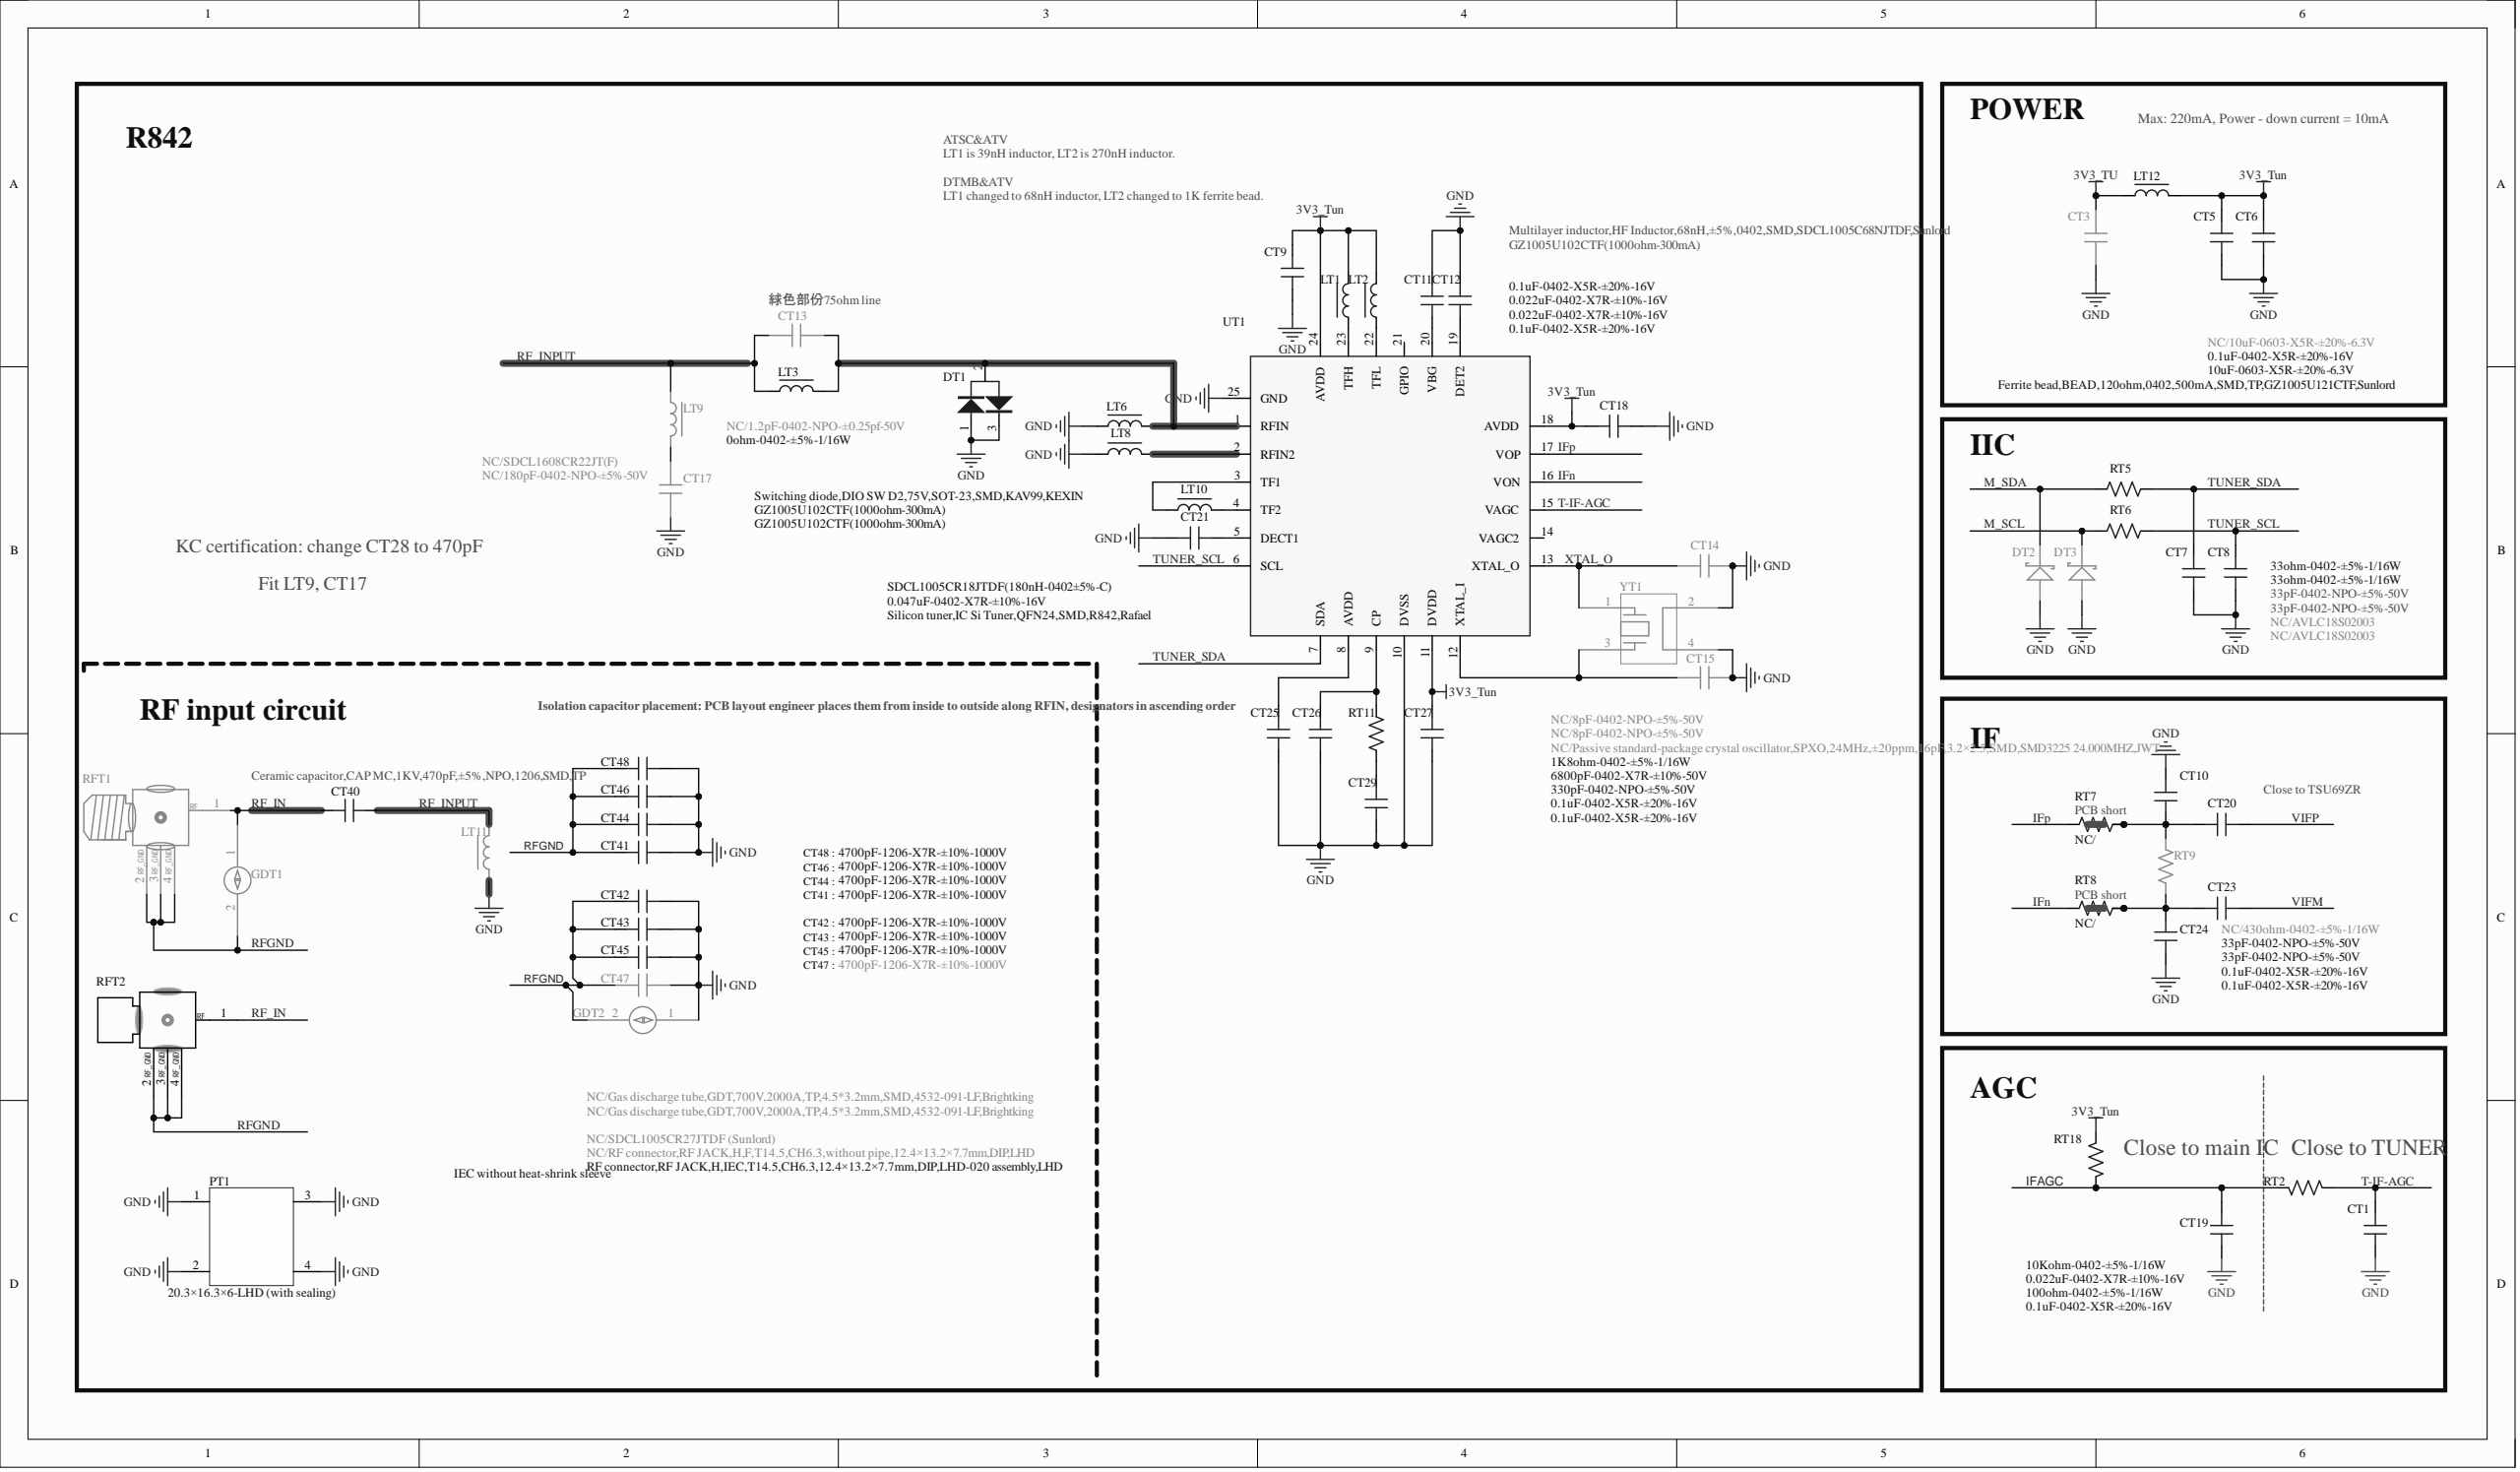Circuit board | Altium Designer | 574 parts | 274 nets | one sheet of the schematic
Parts on this sheet (reference | value | footprint):
CT1 | 0.1uF-0402-X5R-±20%-16V | C0402
CT3 | NC/10uF-0603-X5R-±20%-6.3V | C0603
CT5 | 0.1uF-0402-X5R-±20%-16V | C0402
CT6 | 10uF-0603-X5R-±20%-6.3V | C0603
CT7 | 33pF-0402-NPO-±5%-50V | C0402
CT8 | 33pF-0402-NPO-±5%-50V | C0402
CT9 | 0.1uF-0402-X5R-±20%-16V | C0402
CT10 | 33pF-0402-NPO-±5%-50V | C0402
CT11 | 0.022uF-0402-X7R-±10%-16V | C0402
CT12 | 0.022uF-0402-X7R-±10%-16V | C0402
CT13 | NC/1.2pF-0402-NPO-±0.25pf-50V | C0402
CT14 | NC/8pF-0402-NPO-±5%-50V | C0402
CT15 | NC/8pF-0402-NPO-±5%-50V | C0402
CT17 | NC/180pF-0402-NPO-±5%-50V | C0402
CT18 | 0.1uF-0402-X5R-±20%-16V | C0402
CT19 | 0.022uF-0402-X7R-±10%-16V | C0402
CT20 | 0.1uF-0402-X5R-±20%-16V | C0402
CT21 | 0.047uF-0402-X7R-±10%-16V | C0402
CT23 | 0.1uF-0402-X5R-±20%-16V | C0402
CT24 | 33pF-0402-NPO-±5%-50V | C0402
CT25 | 0.1uF-0402-X5R-±20%-16V | C0402
CT26 | 330pF-0402-NPO-±5%-50V | C0402
CT27 | 0.1uF-0402-X5R-±20%-16V | C0402
CT29 | 6800pF-0402-X7R-±10%-50V | C0402
CT40 | Ceramic capacitor,CAP MC,1KV,470pF,±5%,NPO,1206,SMD,TP | C1206
CT41 | 4700pF-1206-X7R-±10%-1000V | C1206
CT42 | 4700pF-1206-X7R-±10%-1000V | C1206
CT43 | 4700pF-1206-X7R-±10%-1000V | C1206
CT44 | 4700pF-1206-X7R-±10%-1000V | C1206
CT45 | 4700pF-1206-X7R-±10%-1000V | C1206
CT46 | 4700pF-1206-X7R-±10%-1000V | C1206
CT47 | 4700pF-1206-X7R-±10%-1000V | C1206
CT48 | 4700pF-1206-X7R-±10%-1000V | C1206
DT1 | Switching diode,DIO SW D2,75V,SOT-23,SMD,KAV99,KEXIN | SO-23
DT2 | NC/AVLC18S02003 | DIODE-S0402
DT3 | NC/AVLC18S02003 | DIODE-S0402
GDT1 | NC/Gas discharge tube,GDT,700V,2000A,TP,4.5*3.2mm,SMD,4532-091-LF,Brightking | SMD4532-1
GDT2 | NC/Gas discharge tube,GDT,700V,2000A,TP,4.5*3.2mm,SMD,4532-091-LF,Brightking | SMD4532-1
LT1 | Multilayer inductor,HF Inductor,68nH,±5%,0402,SMD,SDCL1005C68NJTDF,Sunlord | L0402
LT2 | GZ1005U102CTF(1000ohm-300mA) | L0402
LT3 | 0ohm-0402-±5%-1/16W | L0402
LT6 | GZ1005U102CTF(1000ohm-300mA) | L0402
LT8 | GZ1005U102CTF(1000ohm-300mA) | L0402
LT9 | NC/SDCL1608CR22JT(F) | L0603
LT10 | SDCL1005CR18JTDF(180nH-0402±5%-C) | L0402
LT11 | NC/SDCL1005CR27JTDF (Sunlord) | L0402
LT12 | Ferrite bead,BEAD,120ohm,0402,500mA,SMD,TP,GZ1005U121CTF,Sunlord | L0402
PT1 | 20.3×16.3×6-LHD (with sealing) | SHIELD(16*20*6)
RFT1 | NC/RF connector,RF JACK,H,F,T14.5,CH6.3,without pipe,12.4×13.2×7.7mm,DIP,LHD | T-13.2×12.4×7.7-F14.5
RFT2 | RF connector,RF JACK,H,IEC,T14.5,CH6.3,12.4×13.2×7.7mm,DIP,LHD-020 assembly,LHD | ANT-IEC14.5-H-4
RT2 | 100ohm-0402-±5%-1/16W | R0402
RT5 | 33ohm-0402-±5%-1/16W | R0402
RT6 | 33ohm-0402-±5%-1/16W | R0402
RT7 | NC/ | R0402SC
RT8 | NC/ | R0402SC
RT9 | NC/430ohm-0402-±5%-1/16W | R0402
RT11 | 1K8ohm-0402-±5%-1/16W | R0402
RT18 | 10Kohm-0402-±5%-1/16W | R0402
UT1 | Silicon tuner,IC Si Tuner,QFN24,SMD,R842,Rafael | QFN24/0.5-3
YT1 | NC/Passive standard-package crystal oscillator,SPXO,24MHz,±20ppm,16pF,3.2×2.5,SMD,SMD3225 24.000MHZ,JWT | XTAL-S-10
Nets of these parts (net: part-pin ...):
XTAL_O: CT14-2 YT1-1 UT1-13
VIFP: CT20-2
VIFM: CT23-2
TUNER_SDA: CT7-2 RT5-2 UT1-7
TUNER_SCL: CT8-2 RT6-2 UT1-6
T-IF-AGC: CT1-2 RT2-1 UT1-15
RFGND: CT41-2 CT42-2 CT43-2 CT44-2 CT45-2 CT46-2 CT47-2 CT48-2 GDT1-2 GDT2-2 RFT1-2 RFT1-3 RFT1-4 RFT2-2 RFT2-3 RFT2-4
RF_INPUT: CT13-1 CT40-2 LT3-1 LT9-1 LT11-1
RF_IN: CT40-1 GDT1-1 RFT1-1 RFT2-1
NetLT10_2: LT10-2 UT1-3
NetLT10_1: LT10-1 UT1-4
NetLT8_1: LT8-1 UT1-2
NetLT2_1: LT2-1 UT1-22
NetLT1_2: LT1-2 UT1-23
NetCT29_2: CT29-2 RT11-1
NetCT26_2: CT26-2 RT11-2 UT1-9
NetCT25_1: CT25-1 UT1-8
NetCT23_1: CT23-1 CT24-2 RT8-2 RT8-3 RT9-2
NetCT21_1: CT21-1 UT1-5
NetCT17_1: CT17-1 LT9-2
NetCT15_2: CT15-2 YT1-3 UT1-12
NetCT13_2: CT13-2 DT1-2 LT3-2 LT6-1 UT1-1
NetCT12_1: CT12-1 UT1-19
NetCT11_2: CT11-2 UT1-20
NetCT10_1: CT10-1 CT20-1 RT7-2 RT7-3 RT9-1
M_SDA: DT2-K RT5-1
M_SCL: DT3-K RT6-1
IFp: RT7-1 UT1-17
IFn: RT8-1 UT1-16
IFAGC: CT19-2 RT2-2 RT18-2
GND: CT1-1 CT3-2 CT5-1 CT6-2 CT7-1 CT8-1 CT9-2 CT10-2 CT11-1 CT12-2 CT14-1 CT15-1 CT17-2 CT18-1 CT19-1 CT21-2 CT24-1 CT25-2 CT26-1 CT27-2 CT29-1 CT41-1 CT42-1 CT43-1 CT44-1 CT45-1 CT46-1 CT47-1 CT48-1 DT1-1 DT1-3 DT2-A DT3-A GDT2-1 LT6-2 LT8-2 LT11-2 PT1-1 PT1-2 PT1-3 PT1-4 YT1-2 YT1-4 UT1-10 UT1-25
3V3_Tun: CT5-2 CT6-1 CT9-1 CT18-2 CT27-1 LT1-1 LT2-2 LT12-2 RT18-1 UT1-11 UT1-18 UT1-24
3V3_TU: CT3-1 LT12-1